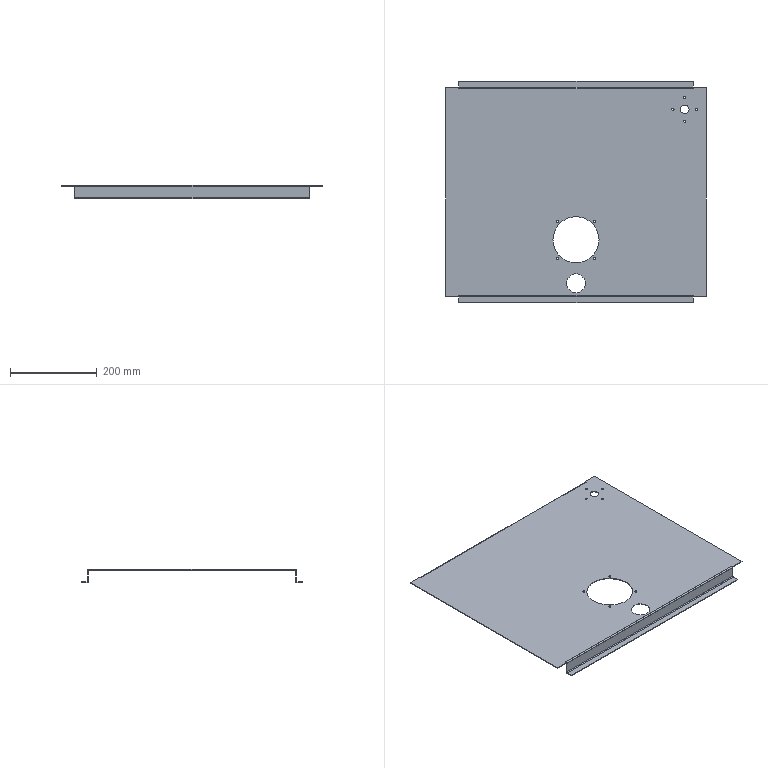Part | SolidWorks | features ICE 3, EdgeFlange 2, FlatPattern 1, SMBaseFlange 1, SheetMetal 1 | 1 solid | 68 faces | box 600 x 510 x 30 mm | volume 483219 mm3 | plane 38 | cylinder 30 | commonest cylinder face diameters 5 x16 3 x4 6 x4 20 x2 43 x2 106 x2